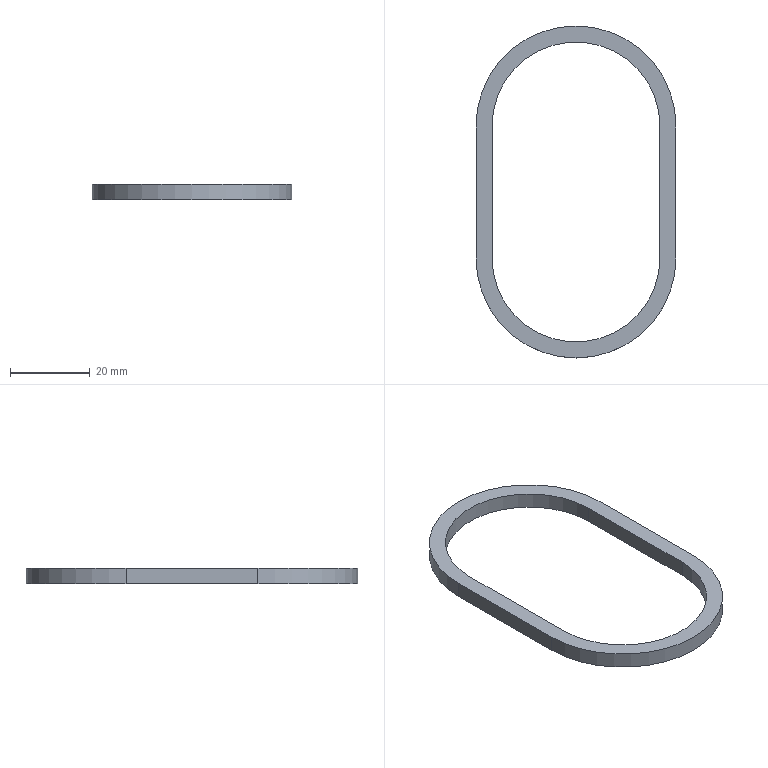Part | SolidWorks | features Extrusion 1 | 1 solid | 10 faces | box 50 x 83 x 4 mm | volume 3368 mm3 | plane 6 | cylinder 4 | commonest cylinder face diameters 42 x2 50 x2
STEP:
#1=CARTESIAN_POINT('',(25.,16.5,4.));
#2=VERTEX_POINT('',#1);
#3=CARTESIAN_POINT('',(-25.,16.5,4.));
#4=VERTEX_POINT('',#3);
#5=CARTESIAN_POINT('',(0.,16.5,4.));
#6=DIRECTION('',(0.,0.,1.));
#7=DIRECTION('',(1.,0.,0.));
#8=AXIS2_PLACEMENT_3D('',#5,#6,#7);
#9=CIRCLE('',#8,25.);
#10=EDGE_CURVE('',#2,#4,#9,.T.);
#11=ORIENTED_EDGE('',*,*,#10,.T.);
#12=CARTESIAN_POINT('',(-25.,-16.5,4.));
#13=VERTEX_POINT('',#12);
#14=CARTESIAN_POINT('',(-25.,16.5,4.));
#15=DIRECTION('',(0.,-1.,0.));
#16=VECTOR('',#15,1000.);
#17=LINE('',#14,#16);
#18=EDGE_CURVE('',#4,#13,#17,.T.);
#19=ORIENTED_EDGE('',*,*,#18,.T.);
#20=CARTESIAN_POINT('',(25.,-16.5,4.));
#21=VERTEX_POINT('',#20);
#22=CARTESIAN_POINT('',(0.,-16.5,4.));
#23=DIRECTION('',(0.,0.,1.));
#24=DIRECTION('',(-1.,0.,0.));
#25=AXIS2_PLACEMENT_3D('',#22,#23,#24);
#26=CIRCLE('',#25,25.);
#27=EDGE_CURVE('',#13,#21,#26,.T.);
#28=ORIENTED_EDGE('',*,*,#27,.T.);
#29=CARTESIAN_POINT('',(25.,16.5,4.));
#30=DIRECTION('',(0.,1.,0.));
#31=VECTOR('',#30,1000.);
#32=LINE('',#29,#31);
#33=EDGE_CURVE('',#21,#2,#32,.T.);
#34=ORIENTED_EDGE('',*,*,#33,.T.);
#35=EDGE_LOOP('',(#11,#19,#28,#34));
#36=FACE_OUTER_BOUND('',#35,.T.);
#37=CARTESIAN_POINT('',(21.,-16.5,4.));
#38=VERTEX_POINT('',#37);
#39=CARTESIAN_POINT('',(21.,16.5,4.));
#40=VERTEX_POINT('',#39);
#41=CARTESIAN_POINT('',(21.,16.5,4.));
#42=DIRECTION('',(0.,1.,0.));
#43=VECTOR('',#42,1000.);
#44=LINE('',#41,#43);
#45=EDGE_CURVE('',#38,#40,#44,.T.);
#46=ORIENTED_EDGE('',*,*,#45,.F.);
#47=CARTESIAN_POINT('',(-21.,-16.5,4.));
#48=VERTEX_POINT('',#47);
#49=CARTESIAN_POINT('',(0.,-16.5,4.));
#50=DIRECTION('',(0.,0.,1.));
#51=DIRECTION('',(-1.,0.,0.));
#52=AXIS2_PLACEMENT_3D('',#49,#50,#51);
#53=CIRCLE('',#52,21.);
#54=EDGE_CURVE('',#48,#38,#53,.T.);
#55=ORIENTED_EDGE('',*,*,#54,.F.);
#56=CARTESIAN_POINT('',(-21.,16.5,4.));
#57=VERTEX_POINT('',#56);
#58=CARTESIAN_POINT('',(-21.,16.5,4.));
#59=DIRECTION('',(0.,-1.,0.));
#60=VECTOR('',#59,1000.);
#61=LINE('',#58,#60);
#62=EDGE_CURVE('',#57,#48,#61,.T.);
#63=ORIENTED_EDGE('',*,*,#62,.F.);
#64=CARTESIAN_POINT('',(0.,16.5,4.));
#65=DIRECTION('',(0.,0.,1.));
#66=DIRECTION('',(1.,0.,0.));
#67=AXIS2_PLACEMENT_3D('',#64,#65,#66);
#68=CIRCLE('',#67,21.);
#69=EDGE_CURVE('',#40,#57,#68,.T.);
#70=ORIENTED_EDGE('',*,*,#69,.F.);
#71=EDGE_LOOP('',(#46,#55,#63,#70));
#72=FACE_BOUND('',#71,.T.);
#73=CARTESIAN_POINT('',(0.,16.5,4.));
#74=DIRECTION('',(0.,0.,1.));
#75=DIRECTION('',(1.,0.,0.));
#76=AXIS2_PLACEMENT_3D('',#73,#74,#75);
#77=PLANE('',#76);
#78=ADVANCED_FACE('',(#36,#72),#77,.T.);
#79=CARTESIAN_POINT('',(25.,16.5,0.));
#80=VERTEX_POINT('',#79);
#81=CARTESIAN_POINT('',(-25.,16.5,0.));
#82=VERTEX_POINT('',#81);
#83=CARTESIAN_POINT('',(0.,16.5,0.));
#84=DIRECTION('',(0.,0.,1.));
#85=DIRECTION('',(1.,0.,0.));
#86=AXIS2_PLACEMENT_3D('',#83,#84,#85);
#87=CIRCLE('',#86,25.);
#88=EDGE_CURVE('',#80,#82,#87,.T.);
#89=ORIENTED_EDGE('',*,*,#88,.F.);
#90=CARTESIAN_POINT('',(25.,-16.5,0.));
#91=VERTEX_POINT('',#90);
#92=CARTESIAN_POINT('',(25.,16.5,0.));
#93=DIRECTION('',(0.,1.,0.));
#94=VECTOR('',#93,1000.);
#95=LINE('',#92,#94);
#96=EDGE_CURVE('',#91,#80,#95,.T.);
#97=ORIENTED_EDGE('',*,*,#96,.F.);
#98=CARTESIAN_POINT('',(-25.,-16.5,0.));
#99=VERTEX_POINT('',#98);
#100=CARTESIAN_POINT('',(0.,-16.5,0.));
#101=DIRECTION('',(0.,0.,1.));
#102=DIRECTION('',(-1.,0.,0.));
#103=AXIS2_PLACEMENT_3D('',#100,#101,#102);
#104=CIRCLE('',#103,25.);
#105=EDGE_CURVE('',#99,#91,#104,.T.);
#106=ORIENTED_EDGE('',*,*,#105,.F.);
#107=CARTESIAN_POINT('',(-25.,16.5,0.));
#108=DIRECTION('',(0.,-1.,0.));
#109=VECTOR('',#108,1000.);
#110=LINE('',#107,#109);
#111=EDGE_CURVE('',#82,#99,#110,.T.);
#112=ORIENTED_EDGE('',*,*,#111,.F.);
#113=EDGE_LOOP('',(#89,#97,#106,#112));
#114=FACE_OUTER_BOUND('',#113,.T.);
#115=CARTESIAN_POINT('',(-21.,-16.5,0.));
#116=VERTEX_POINT('',#115);
#117=CARTESIAN_POINT('',(21.,-16.5,0.));
#118=VERTEX_POINT('',#117);
#119=CARTESIAN_POINT('',(0.,-16.5,0.));
#120=DIRECTION('',(0.,0.,1.));
#121=DIRECTION('',(-1.,0.,0.));
#122=AXIS2_PLACEMENT_3D('',#119,#120,#121);
#123=CIRCLE('',#122,21.);
#124=EDGE_CURVE('',#116,#118,#123,.T.);
#125=ORIENTED_EDGE('',*,*,#124,.T.);
#126=CARTESIAN_POINT('',(21.,16.5,0.));
#127=VERTEX_POINT('',#126);
#128=CARTESIAN_POINT('',(21.,16.5,0.));
#129=DIRECTION('',(0.,1.,0.));
#130=VECTOR('',#129,1000.);
#131=LINE('',#128,#130);
#132=EDGE_CURVE('',#118,#127,#131,.T.);
#133=ORIENTED_EDGE('',*,*,#132,.T.);
#134=CARTESIAN_POINT('',(-21.,16.5,0.));
#135=VERTEX_POINT('',#134);
#136=CARTESIAN_POINT('',(0.,16.5,0.));
#137=DIRECTION('',(0.,0.,1.));
#138=DIRECTION('',(1.,0.,0.));
#139=AXIS2_PLACEMENT_3D('',#136,#137,#138);
#140=CIRCLE('',#139,21.);
#141=EDGE_CURVE('',#127,#135,#140,.T.);
#142=ORIENTED_EDGE('',*,*,#141,.T.);
#143=CARTESIAN_POINT('',(-21.,16.5,0.));
#144=DIRECTION('',(0.,-1.,0.));
#145=VECTOR('',#144,1000.);
#146=LINE('',#143,#145);
#147=EDGE_CURVE('',#135,#116,#146,.T.);
#148=ORIENTED_EDGE('',*,*,#147,.T.);
#149=EDGE_LOOP('',(#125,#133,#142,#148));
#150=FACE_BOUND('',#149,.T.);
#151=CARTESIAN_POINT('',(0.,16.5,0.));
#152=DIRECTION('',(0.,0.,1.));
#153=DIRECTION('',(1.,0.,0.));
#154=AXIS2_PLACEMENT_3D('',#151,#152,#153);
#155=PLANE('',#154);
#156=ADVANCED_FACE('',(#114,#150),#155,.F.);
#157=ORIENTED_EDGE('',*,*,#88,.T.);
#158=CARTESIAN_POINT('',(-25.,16.5,4.));
#159=DIRECTION('',(0.,0.,-1.));
#160=VECTOR('',#159,1000.);
#161=LINE('',#158,#160);
#162=EDGE_CURVE('',#4,#82,#161,.T.);
#163=ORIENTED_EDGE('',*,*,#162,.F.);
#164=ORIENTED_EDGE('',*,*,#10,.F.);
#165=CARTESIAN_POINT('',(25.,16.5,4.));
#166=DIRECTION('',(0.,0.,-1.));
#167=VECTOR('',#166,1000.);
#168=LINE('',#165,#167);
#169=EDGE_CURVE('',#2,#80,#168,.T.);
#170=ORIENTED_EDGE('',*,*,#169,.T.);
#171=EDGE_LOOP('',(#157,#163,#164,#170));
#172=FACE_OUTER_BOUND('',#171,.T.);
#173=CARTESIAN_POINT('',(0.,16.5,4.));
#174=DIRECTION('',(0.,0.,-1.));
#175=DIRECTION('',(-1.,0.,0.));
#176=AXIS2_PLACEMENT_3D('',#173,#174,#175);
#177=CYLINDRICAL_SURFACE('',#176,25.);
#178=ADVANCED_FACE('',(#172),#177,.T.);
#179=ORIENTED_EDGE('',*,*,#111,.T.);
#180=CARTESIAN_POINT('',(-25.,-16.5,4.));
#181=DIRECTION('',(0.,0.,-1.));
#182=VECTOR('',#181,1000.);
#183=LINE('',#180,#182);
#184=EDGE_CURVE('',#13,#99,#183,.T.);
#185=ORIENTED_EDGE('',*,*,#184,.F.);
#186=ORIENTED_EDGE('',*,*,#18,.F.);
#187=ORIENTED_EDGE('',*,*,#162,.T.);
#188=EDGE_LOOP('',(#179,#185,#186,#187));
#189=FACE_OUTER_BOUND('',#188,.T.);
#190=CARTESIAN_POINT('',(-25.,16.5,4.));
#191=DIRECTION('',(1.,0.,0.));
#192=DIRECTION('',(0.,0.,-1.));
#193=AXIS2_PLACEMENT_3D('',#190,#191,#192);
#194=PLANE('',#193);
#195=ADVANCED_FACE('',(#189),#194,.F.);
#196=ORIENTED_EDGE('',*,*,#105,.T.);
#197=CARTESIAN_POINT('',(25.,-16.5,4.));
#198=DIRECTION('',(0.,0.,-1.));
#199=VECTOR('',#198,1000.);
#200=LINE('',#197,#199);
#201=EDGE_CURVE('',#21,#91,#200,.T.);
#202=ORIENTED_EDGE('',*,*,#201,.F.);
#203=ORIENTED_EDGE('',*,*,#27,.F.);
#204=ORIENTED_EDGE('',*,*,#184,.T.);
#205=EDGE_LOOP('',(#196,#202,#203,#204));
#206=FACE_OUTER_BOUND('',#205,.T.);
#207=CARTESIAN_POINT('',(0.,-16.5,4.));
#208=DIRECTION('',(0.,0.,-1.));
#209=DIRECTION('',(-1.,0.,0.));
#210=AXIS2_PLACEMENT_3D('',#207,#208,#209);
#211=CYLINDRICAL_SURFACE('',#210,25.);
#212=ADVANCED_FACE('',(#206),#211,.T.);
#213=ORIENTED_EDGE('',*,*,#96,.T.);
#214=ORIENTED_EDGE('',*,*,#169,.F.);
#215=ORIENTED_EDGE('',*,*,#33,.F.);
#216=ORIENTED_EDGE('',*,*,#201,.T.);
#217=EDGE_LOOP('',(#213,#214,#215,#216));
#218=FACE_OUTER_BOUND('',#217,.T.);
#219=CARTESIAN_POINT('',(25.,16.5,4.));
#220=DIRECTION('',(-1.,0.,0.));
#221=DIRECTION('',(0.,0.,1.));
#222=AXIS2_PLACEMENT_3D('',#219,#220,#221);
#223=PLANE('',#222);
#224=ADVANCED_FACE('',(#218),#223,.F.);
#225=ORIENTED_EDGE('',*,*,#124,.F.);
#226=CARTESIAN_POINT('',(-21.,-16.5,4.));
#227=DIRECTION('',(0.,0.,-1.));
#228=VECTOR('',#227,1000.);
#229=LINE('',#226,#228);
#230=EDGE_CURVE('',#48,#116,#229,.T.);
#231=ORIENTED_EDGE('',*,*,#230,.F.);
#232=ORIENTED_EDGE('',*,*,#54,.T.);
#233=CARTESIAN_POINT('',(21.,-16.5,4.));
#234=DIRECTION('',(0.,0.,-1.));
#235=VECTOR('',#234,1000.);
#236=LINE('',#233,#235);
#237=EDGE_CURVE('',#38,#118,#236,.T.);
#238=ORIENTED_EDGE('',*,*,#237,.T.);
#239=EDGE_LOOP('',(#225,#231,#232,#238));
#240=FACE_OUTER_BOUND('',#239,.T.);
#241=CARTESIAN_POINT('',(0.,-16.5,4.));
#242=DIRECTION('',(0.,0.,-1.));
#243=DIRECTION('',(-1.,0.,0.));
#244=AXIS2_PLACEMENT_3D('',#241,#242,#243);
#245=CYLINDRICAL_SURFACE('',#244,21.);
#246=ADVANCED_FACE('',(#240),#245,.F.);
#247=ORIENTED_EDGE('',*,*,#132,.F.);
#248=ORIENTED_EDGE('',*,*,#237,.F.);
#249=ORIENTED_EDGE('',*,*,#45,.T.);
#250=CARTESIAN_POINT('',(21.,16.5,4.));
#251=DIRECTION('',(0.,0.,-1.));
#252=VECTOR('',#251,1000.);
#253=LINE('',#250,#252);
#254=EDGE_CURVE('',#40,#127,#253,.T.);
#255=ORIENTED_EDGE('',*,*,#254,.T.);
#256=EDGE_LOOP('',(#247,#248,#249,#255));
#257=FACE_OUTER_BOUND('',#256,.T.);
#258=CARTESIAN_POINT('',(21.,16.5,4.));
#259=DIRECTION('',(-1.,0.,0.));
#260=DIRECTION('',(0.,0.,1.));
#261=AXIS2_PLACEMENT_3D('',#258,#259,#260);
#262=PLANE('',#261);
#263=ADVANCED_FACE('',(#257),#262,.T.);
#264=ORIENTED_EDGE('',*,*,#141,.F.);
#265=ORIENTED_EDGE('',*,*,#254,.F.);
#266=ORIENTED_EDGE('',*,*,#69,.T.);
#267=CARTESIAN_POINT('',(-21.,16.5,4.));
#268=DIRECTION('',(0.,0.,-1.));
#269=VECTOR('',#268,1000.);
#270=LINE('',#267,#269);
#271=EDGE_CURVE('',#57,#135,#270,.T.);
#272=ORIENTED_EDGE('',*,*,#271,.T.);
#273=EDGE_LOOP('',(#264,#265,#266,#272));
#274=FACE_OUTER_BOUND('',#273,.T.);
#275=CARTESIAN_POINT('',(0.,16.5,4.));
#276=DIRECTION('',(0.,0.,-1.));
#277=DIRECTION('',(-1.,0.,0.));
#278=AXIS2_PLACEMENT_3D('',#275,#276,#277);
#279=CYLINDRICAL_SURFACE('',#278,21.);
#280=ADVANCED_FACE('',(#274),#279,.F.);
#281=ORIENTED_EDGE('',*,*,#147,.F.);
#282=ORIENTED_EDGE('',*,*,#271,.F.);
#283=ORIENTED_EDGE('',*,*,#62,.T.);
#284=ORIENTED_EDGE('',*,*,#230,.T.);
#285=EDGE_LOOP('',(#281,#282,#283,#284));
#286=FACE_OUTER_BOUND('',#285,.T.);
#287=CARTESIAN_POINT('',(-21.,16.5,4.));
#288=DIRECTION('',(1.,0.,0.));
#289=DIRECTION('',(0.,1.,0.));
#290=AXIS2_PLACEMENT_3D('',#287,#288,#289);
#291=PLANE('',#290);
#292=ADVANCED_FACE('',(#286),#291,.T.);
#293=CLOSED_SHELL('',(#78,#156,#178,#195,#212,#224,#246,#263,#280,#292));
#294=MANIFOLD_SOLID_BREP('',#293);
#295=CARTESIAN_POINT('',(0.,0.,0.));
#296=DIRECTION('',(0.,0.,1.));
#297=DIRECTION('',(1.,0.,0.));
#298=AXIS2_PLACEMENT_3D('',#295,#296,#297);
#299=(LENGTH_UNIT()NAMED_UNIT(*)SI_UNIT(.MILLI.,.METRE.));
#300=UNCERTAINTY_MEASURE_WITH_UNIT(LENGTH_MEASURE(0.00001),#299,'','');
#301=(NAMED_UNIT(*)PLANE_ANGLE_UNIT()SI_UNIT($,.RADIAN.));
#302=(NAMED_UNIT(*)SI_UNIT($,.STERADIAN.)SOLID_ANGLE_UNIT());
#303=(GEOMETRIC_REPRESENTATION_CONTEXT(3)GLOBAL_UNCERTAINTY_ASSIGNED_CONTEXT((#300))GLOBAL_UNIT_ASSIGNED_CONTEXT((#299,#301,#302))REPRESENTATION_CONTEXT('',''));
#304=ADVANCED_BREP_SHAPE_REPRESENTATION('',(#294,#298),#303);